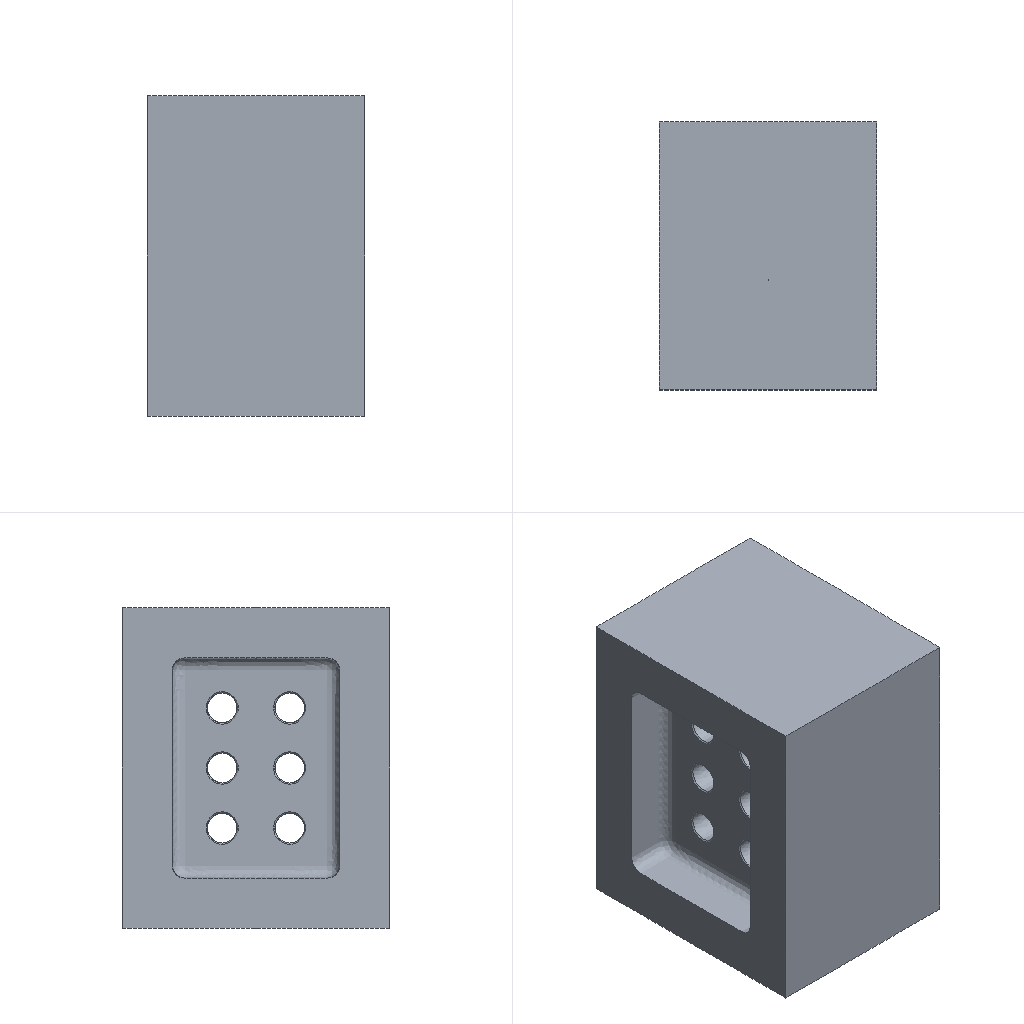Simulation study | ansys workbench
Set-up summary:
category,name,step,type,value,unit,region
solver,ansys_workbench
units,mm-N-s-tonne (MPa),,stated,"/units,MPA"
analysis,LS1,,static
load_step,LS1,LS1,static,nsubst=1; time=1
load_step,LS2,LS2,static,nsubst=1; time=2
mesh,nodes,,,452829
mesh,elements,,,327929
element_type,SOLID187,,,303965
element_type,CONTA174,,,10988
element_type,TARGE170,,,10076
element_type,SURF154,,,2900
material,Structural Steel,,E,200000,tonne s^-2 mm^-1
material,Structural Steel,,nu,0.3
material,Structural Steel,,density,7.85e-09,tonne mm^-3
material,Structural Steel,,conductivity,60.5,tonne mm s^-3 C^-1
material,Structural Steel,,specific_heat,4.34e+08,mm^2 s^-2 C^-1
material,Structural Steel,,cte,1.2e-05,C^-1
material,Structural Steel,,permeability,10000
material,Structural Steel,,resistivity,0.00017,ohm mm
material,mat 29,,E,200000,tonne s^-2 mm^-1
material,mat 29,,nu,0.3
material,mat 29,,density,7.85e-09,tonne mm^-3
material,mat 29,,conductivity,60.5,tonne mm s^-3 C^-1
material,mat 29,,specific_heat,4.34e+08,mm^2 s^-2 C^-1
material,mat 29,,cte,1.2e-05,C^-1
material,mat 29,,permeability,10000
material,mat 29,,resistivity,0.00017,ohm mm
load,Define Force Using Surface Effect Elements,LS1,surface-effect pres face 1,-0.1279,,SURF154 #35
load,Define Force Using Surface Effect Elements,LS1,surface-effect pres face 2,1.43512e-17,,SURF154 #35
load,Define Force Using Surface Effect Elements,LS1,surface-effect pres face 3,6.77494e-18,,SURF154 #35
load,,LS1,force,"6000 [dir=(1, 0, 0) n=6]",,node list
bc,Fixed Supports,model,fixed,[dofs=ALL],,_FIXEDSU
bc,,LS2,prescribed ux,table _FIX [dofs=UX n=6],,node list
contact,Frictional - ? ? ?,,standard (frictionless/frictional),friction=0.2; element=CONTA174
contact,contact 2,,bonded (always),element=CONTA174
contact,contact 3,,bonded (always),element=CONTA174
contact,contact 4,,bonded (always),element=CONTA174
contact,contact 5,,bonded (always),element=CONTA174
contact,contact 6,,bonded (always),element=CONTA174
contact,contact 7,,bonded (always),element=CONTA174
contact,contact 8,,bonded (always),element=CONTA174
contact,contact 9,,bonded (always),element=CONTA174
contact,contact 10,,bonded (always),element=CONTA174
contact,contact 11,,bonded (always),element=CONTA174
contact,contact 12,,bonded (always),element=CONTA174
contact,contact 13,,bonded (always),element=CONTA174
named_set,_FIXEDSU,,node,6188
Ansys APDL input file, long lists of numbers shortened:
/batch
/config,noeldb,1     ! force off writing results to database
*get,_wallstrt,active,,time,wall
! ANSYS input file written by Workbench version 2021 R1
! File used for geometry attach:
/title,__--____ (B5)
! ****** Begin Custom Load Command Snippet ******
/COM, ACT Extensions:
/COM,     LSDYNA, 2021.1
/COM,
! ****** End   Custom Load Command Snippet ******
*DIM,_wb_ProjectScratch_dir,string,248
_wb_ProjectScratch_dir(1) = ''
*DIM,_wb_SolverFiles_dir,string,248
_wb_SolverFiles_dir(1) = ''
*DIM,_wb_userfiles_dir,string,248
_wb_userfiles_dir(1) = ''
/com,--- Data in consistent NMM units. See Solving Units in the help system for more information.
/units,MPA
/nopr
/wb,file,start              !  signify a WB generated input file
/prep7
! Turn off shape checking because checks already performed inside WB mesher.
! See help system for more information.
SHPP,OFF,,NOWARN
/nolist
etcon,set             ! allow ANSYS to choose best KEYOP's for 180x elements, resets any applicable keyopt to MAPDL defaults
/com,*********** Nodes for the whole assembly ***********
nblock,3,,498092
(1i9,3e20.9e3)
        1     2.300000000E+01     1.350000000E+01     7.150000000E+01
! (452810 more lines like these left out)
-1
/com,*********** Nodes for all Remote Points ***********
nblock,3
(1i9,3e20.9e3)
   452812    -2.349999920E+01     1.350120327E+01     6.550000084E+01
! (17 more lines like these left out)
-1
/wb,elem,start            !  set before creation of elements
/com,*********** Elements for Body 1 "__" ***********
et,1,187
eblock,19,solid,,152287
(19i9)
        1        1        1        1        0        0        0        0       10        0   151679   245149   257424   247867   249921   386975   405592   386966   386970
! (304573 more lines like these left out)
-1
/com,*********** Elements for Body 2 "__" ***********
et,2,187
eblock,19,solid,,151678
(19i9)
        2        2        2        2        0        0        0        0       10        0        1    15184    18821    31336    21045   135985   158937   135991   135988
! (303355 more lines like these left out)
-1
/wb,elem,end               !  done creating elements
/com,*********** Send User Defined Coordinate System(s) ***********
csys,0
toffst,273.15,  ! Temperature offset from absolute zero
/com,*********** Set Reference Temperature ***********
tref,22.
/wb,mat,start              !  starting to send materials
/com,*********** Send Materials ***********
Temperature = 'TEMP' ! Temperature
MP,DENS,1,7.85e-09,	! tonne mm^-3
MP,ALPX,1,1.2e-05,	! C^-1
MP,C,1,434000000,	! mm^2 s^-2 C^-1
MP,KXX,1,60.5,	! tonne mm s^-3 C^-1
MP,RSVX,1,0.00017,	! ohm mm
MP,EX,1,200000,	! tonne s^-2 mm^-1
MP,NUXY,1,0.3,
MP,MURX,1,10000,
Temperature = 'TEMP' ! Temperature
MP,DENS,2,7.85e-09,	! tonne mm^-3
MP,ALPX,2,1.2e-05,	! C^-1
MP,C,2,434000000,	! mm^2 s^-2 C^-1
MP,KXX,2,60.5,	! tonne mm s^-3 C^-1
MP,RSVX,2,0.00017,	! ohm mm
MP,EX,2,200000,	! tonne s^-2 mm^-1
MP,NUXY,2,0.3,
MP,MURX,2,10000,
/wb,mat,end                !  done sending materials
!************************* Model Summary ********************
!__,	结构钢,	matid,	1
!__,	结构钢,	matid,	2
!************************* End Model Summary ********************
! get the diagonal of the bounding box. Needed later for other things
*get,_xmin,node,,mnloc,x
*get,_ymin,node,,mnloc,y
*get,_zmin,node,,mnloc,z
*get,_xmax,node,,mxloc,x
*get,_ymax,node,,mxloc,y
*get,_zmax,node,,mxloc,z
_ASMDIAG=(_xmax-_xmin)*(_xmax-_xmin)+(_ymax-_ymin)*(_ymax-_ymin)+(_zmax-_zmin)*(_zmax-_zmin)
_ASMDIAG=SQRT(_ASMDIAG)
/wb,contact,start          !  starting to send contact
/com,*********** Create Contact "摩擦的 - 固体 至 固体" ***********
/com,            Real Constant Set For Above Contact Is 4 & 3
*set,tid,4
*set,cid,3
r,tid
r,cid
et,tid,170
et,cid,174
eblock,10,,,5038
(15i9)
   350529        4        4        4        0   230477   230549   229930   229930   289067   283934   229930   283933
! (5037 more lines like these left out)
-1
eblock,10,,,5038
(15i9)
   355567        3        3        3        0   230477   230549   229930   229930   289067   283934   229930   283933
! (5037 more lines like these left out)
-1
eblock,10,,,5038
(15i9)
   360605        3        4        3        0     3593     4585     4192     4192    56241    61610     4192    56239
! (5037 more lines like these left out)
-1
eblock,10,,,5038
(15i9)
   365643        4        3        4        0     3593     4585     4192     4192    56241    61610     4192    56239
! (5037 more lines like these left out)
-1
keyo,cid,8,2               ! auto create asymmetric contact (from Program Controlled setting)
keyo,cid,10,0              ! adjust contact stiffness each NR iteration (from Program Controlled setting)
keyo,cid,12,0              ! standard contact
mp,mu,cid,0.2       ! unitless
keyo,cid,18,1              ! small sliding turned on by application
keyo,cid,2,0               ! augmented Lagrange (from Program Controlled setting)
keyo,cid,4,0               ! on Gauss point (from Program Controlled setting)
keyo,cid,9,0               ! use real geometry with stepped effects
keyo,cid,7,0               ! No Prediction
rmod,tid,3,1.       ! FKN
rmod,tid,5,0.       ! ICONT
rmod,tid,6,0.       ! PINB
rmod,tid,10,0.      ! CNOF
rmod,tid,12,0.      ! FKT
rmod,tid,36,27      ! WB DSID
rmod,cid,3,1.       ! FKN
rmod,cid,5,0.       ! ICONT
rmod,cid,6,0.       ! PINB
rmod,cid,10,0.      ! CNOF
rmod,cid,12,0.      ! FKT
rmod,cid,36,27      ! WB DSID
nsel,all
esel,all
/wb,contact,end            !  done creating contacts
/golist
/wb,load,start             !  starting to send loads
/com,*********** Fixed Supports ***********
CMBLOCK,_FIXEDSU,NODE,     6188
(8i10)
      1057      1079      1080      1081      1082      1083      1084      1085
! (773 more lines like these left out)
cmsel,s,_FIXEDSU
d,all,all
nsel,all
/com,*********** Create Remote Point "内部远程点" ***********
! -------- Remote Point Used by "循环的 - 固体 至 固体" --------
*set,tid,6
*set,cid,5
et,cid,174
et,tid,170
keyo,tid,2,1               ! Don't fix the pilot node
keyo,tid,4,111111
keyo,cid,12,5              ! Bonded Contact
keyo,cid,4,2               ! Rigid CERIG style load
keyo,cid,2,2               ! MPC style contact
eblock,10,,,64
(15i9)
   370681        5        5        5        0   226617   226628   226629   226629   262476   262567   226629   262477
! (63 more lines like these left out)
-1
*set,_npilot,452812
_npilot40=_npilot
type,tid
mat ,cid
real,cid
tshape,pilo
en,370745,_npilot
tshape
/com,*********** Create Remote Point "内部远程点 2" ***********
! -------- Remote Point Used by "循环的 - 固体 至 固体" --------
*set,tid,8
*set,cid,7
et,cid,174
et,tid,170
keyo,tid,2,1               ! Don't fix the pilot node
keyo,tid,4,111111
keyo,cid,12,5              ! Bonded Contact
keyo,cid,4,2               ! Rigid CERIG style load
keyo,cid,2,2               ! MPC style contact
eblock,10,,,88
(15i9)
   370746        7        7        7        0       20       21     7441     7441    31465    31471     7441    31466
! (87 more lines like these left out)
-1
*set,_npilot,452813
_npilot41=_npilot
type,tid
mat ,cid
real,cid
tshape,pilo
en,370834,_npilot
tshape
/com,*********** Create Remote Point "内部远程点" ***********
! -------- Remote Point Used by "循环的 - 固体 至 固体" --------
*set,tid,10
*set,cid,9
et,cid,174
et,tid,170
keyo,tid,2,1               ! Don't fix the pilot node
keyo,tid,4,111111
keyo,cid,12,5              ! Bonded Contact
keyo,cid,4,2               ! Rigid CERIG style load
keyo,cid,2,2               ! MPC style contact
eblock,10,,,64
(15i9)
   370835        9        9        9        0   226058   226059   226452   226452   257957   257964   226452   257958
! (63 more lines like these left out)
-1
*set,_npilot,452814
_npilot45=_npilot
type,tid
mat ,cid
real,cid
tshape,pilo
en,370899,_npilot
tshape
/com,*********** Create Remote Point "内部远程点 2" ***********
! -------- Remote Point Used by "循环的 - 固体 至 固体" --------
*set,tid,12
*set,cid,11
et,cid,174
et,tid,170
keyo,tid,2,1               ! Don't fix the pilot node
keyo,tid,4,111111
keyo,cid,12,5              ! Bonded Contact
keyo,cid,4,2               ! Rigid CERIG style load
keyo,cid,2,2               ! MPC style contact
eblock,10,,,88
(15i9)
   370900       11       11       11        0      580      701      702      702    35914    36847      702    35915
! (87 more lines like these left out)
-1
*set,_npilot,452815
_npilot47=_npilot
type,tid
mat ,cid
real,cid
tshape,pilo
en,370988,_npilot
tshape
/com,*********** Create Remote Point "内部远程点" ***********
! -------- Remote Point Used by "循环的 - 固体 至 固体" --------
*set,tid,14
*set,cid,13
et,cid,174
et,tid,170
keyo,tid,2,1               ! Don't fix the pilot node
keyo,tid,4,111111
keyo,cid,12,5              ! Bonded Contact
keyo,cid,4,2               ! Rigid CERIG style load
keyo,cid,2,2               ! MPC style contact
eblock,10,,,64
(15i9)
   370989       13       13       13        0   226587   233496   226648   226648   262228   262683   226648   262224
! (63 more lines like these left out)
-1
*set,_npilot,452816
_npilot50=_npilot
type,tid
mat ,cid
real,cid
tshape,pilo
en,371053,_npilot
tshape
/com,*********** Create Remote Point "内部远程点 2" ***********
! -------- Remote Point Used by "循环的 - 固体 至 固体" --------
*set,tid,16
*set,cid,15
et,cid,174
et,tid,170
keyo,tid,2,1               ! Don't fix the pilot node
keyo,tid,4,111111
keyo,cid,12,5              ! Bonded Contact
keyo,cid,4,2               ! Rigid CERIG style load
keyo,cid,2,2               ! MPC style contact
eblock,10,,,88
(15i9)
   371054       15       15       15        0      533      535     7402     7402    35498    35520     7402    35503
! (87 more lines like these left out)
-1
*set,_npilot,452817
_npilot52=_npilot
type,tid
mat ,cid
real,cid
tshape,pilo
en,371142,_npilot
tshape
/com,*********** Create Remote Point "内部远程点" ***********
! -------- Remote Point Used by "循环的 - 固体 至 固体" --------
*set,tid,18
*set,cid,17
et,cid,174
et,tid,170
keyo,tid,2,1               ! Don't fix the pilot node
keyo,tid,4,111111
keyo,cid,12,5              ! Bonded Contact
keyo,cid,4,2               ! Rigid CERIG style load
keyo,cid,2,2               ! MPC style contact
eblock,10,,,64
(15i9)
   371143       17       17       17        0   225993   225994   226486   226486   257544   257552   226486   257545
! (63 more lines like these left out)
-1
*set,_npilot,452818
_npilot55=_npilot
type,tid
mat ,cid
real,cid
tshape,pilo
en,371207,_npilot
tshape
/com,*********** Create Remote Point "内部远程点 2" ***********
! -------- Remote Point Used by "循环的 - 固体 至 固体" --------
*set,tid,20
*set,cid,19
et,cid,174
et,tid,170
keyo,tid,2,1               ! Don't fix the pilot node
keyo,tid,4,111111
keyo,cid,12,5              ! Bonded Contact
keyo,cid,4,2               ! Rigid CERIG style load
keyo,cid,2,2               ! MPC style contact
eblock,10,,,88
(15i9)
   371208       19       19       19        0      606      607     7452     7452    36138    36148     7452    36141
! (87 more lines like these left out)
-1
*set,_npilot,452819
_npilot57=_npilot
type,tid
mat ,cid
real,cid
tshape,pilo
en,371296,_npilot
tshape
/com,*********** Create Remote Point "内部远程点" ***********
! -------- Remote Point Used by "循环的 - 固体 至 固体" --------
*set,tid,22
*set,cid,21
et,cid,174
et,tid,170
keyo,tid,2,1               ! Don't fix the pilot node
keyo,tid,4,111111
keyo,cid,12,5              ! Bonded Contact
keyo,cid,4,2               ! Rigid CERIG style load
keyo,cid,2,2               ! MPC style contact
eblock,10,,,64
(15i9)
   371297       21       21       21        0   226560   226673   226674   226674   262007   262820   226674   262008
! (63 more lines like these left out)
-1
*set,_npilot,452820
_npilot60=_npilot
type,tid
mat ,cid
real,cid
tshape,pilo
en,371361,_npilot
tshape
/com,*********** Create Remote Point "内部远程点 2" ***********
! -------- Remote Point Used by "循环的 - 固体 至 固体" --------
*set,tid,24
*set,cid,23
et,cid,174
et,tid,170
keyo,tid,2,1               ! Don't fix the pilot node
keyo,tid,4,111111
keyo,cid,12,5              ! Bonded Contact
keyo,cid,4,2               ! Rigid CERIG style load
keyo,cid,2,2               ! MPC style contact
eblock,10,,,88
(15i9)
   371362       23       23       23        0      490      672     7471     7471    35135    36672     7471    35139
! (87 more lines like these left out)
-1
*set,_npilot,452821
_npilot62=_npilot
type,tid
mat ,cid
real,cid
tshape,pilo
en,371450,_npilot
tshape
/com,*********** Create Remote Point "内部远程点" ***********
! -------- Remote Point Used by "循环的 - 固体 至 固体" --------
*set,tid,26
*set,cid,25
et,cid,174
et,tid,170
keyo,tid,2,1               ! Don't fix the pilot node
keyo,tid,4,111111
keyo,cid,12,5              ! Bonded Contact
keyo,cid,4,2               ! Rigid CERIG style load
keyo,cid,2,2               ! MPC style contact
eblock,10,,,64
(15i9)
   371451       25       25       25        0   226086   226515   226516   226516   258132   261632   226516   258133
! (63 more lines like these left out)
-1
*set,_npilot,452822
_npilot65=_npilot
type,tid
mat ,cid
real,cid
tshape,pilo
en,371515,_npilot
tshape
/com,*********** Create Remote Point "内部远程点 2" ***********
! -------- Remote Point Used by "循环的 - 固体 至 固体" --------
*set,tid,28
*set,cid,27
et,cid,174
et,tid,170
keyo,tid,2,1               ! Don't fix the pilot node
keyo,tid,4,111111
keyo,cid,12,5              ! Bonded Contact
keyo,cid,4,2               ! Rigid CERIG style load
keyo,cid,2,2               ! MPC style contact
eblock,10,,,88
(15i9)
   371516       27       27       27        0      651     7490      653      653    36542    36557      653    36537
! (87 more lines like these left out)
-1
*set,_npilot,452823
_npilot67=_npilot
type,tid
mat ,cid
real,cid
tshape,pilo
en,371604,_npilot
tshape
/com,*********** Create Beam Connection "___ - __ _ __" ***********
/com,            Real Constant Set For Above Beam Connection Is 29
*set,_bid,29
et,_bid,188
mat,_bid
real,_bid
type,_bid
secnum,_bid
en,350497,452812,452813
sectype,29,beam,csolid
secdata,5.
secoffset,cent
Temperature = 'TEMP' ! Temperature
MP,DENS,29,7.85e-09,	! tonne mm^-3
MP,ALPX,29,1.2e-05,	! C^-1
MP,C,29,434000000,	! mm^2 s^-2 C^-1
MP,KXX,29,60.5,	! tonne mm s^-3 C^-1
MP,RSVX,29,0.00017,	! ohm mm
MP,EX,29,200000,	! tonne s^-2 mm^-1
MP,NUXY,29,0.3,
MP,MURX,29,10000,
/com,*********** Create Beam Connection "___ - __ _ __" ***********
/com,            Real Constant Set For Above Beam Connection Is 30
*set,_bid,30
et,_bid,188
mat,_bid
real,_bid
type,_bid
secnum,_bid
en,350502,452814,452815
sectype,30,beam,csolid
secdata,5.
secoffset,cent
Temperature = 'TEMP' ! Temperature
MP,DENS,30,7.85e-09,	! tonne mm^-3
MP,ALPX,30,1.2e-05,	! C^-1
MP,C,30,434000000,	! mm^2 s^-2 C^-1
MP,KXX,30,60.5,	! tonne mm s^-3 C^-1
MP,RSVX,30,0.00017,	! ohm mm
MP,EX,30,200000,	! tonne s^-2 mm^-1
MP,NUXY,30,0.3,
MP,MURX,30,10000,
/com,*********** Create Beam Connection "___ - __ _ __" ***********
/com,            Real Constant Set For Above Beam Connection Is 31
*set,_bid,31
et,_bid,188
mat,_bid
real,_bid
type,_bid
secnum,_bid
en,350507,452816,452817
sectype,31,beam,csolid
secdata,5.
secoffset,cent
Temperature = 'TEMP' ! Temperature
MP,DENS,31,7.85e-09,	! tonne mm^-3
MP,ALPX,31,1.2e-05,	! C^-1
MP,C,31,434000000,	! mm^2 s^-2 C^-1
MP,KXX,31,60.5,	! tonne mm s^-3 C^-1
MP,RSVX,31,0.00017,	! ohm mm
MP,EX,31,200000,	! tonne s^-2 mm^-1
MP,NUXY,31,0.3,
MP,MURX,31,10000,
/com,*********** Create Beam Connection "___ - __ _ __" ***********
/com,            Real Constant Set For Above Beam Connection Is 32
*set,_bid,32
et,_bid,188
mat,_bid
real,_bid
type,_bid
secnum,_bid
en,350512,452818,452819
sectype,32,beam,csolid
secdata,5.
secoffset,cent
Temperature = 'TEMP' ! Temperature
MP,DENS,32,7.85e-09,	! tonne mm^-3
MP,ALPX,32,1.2e-05,	! C^-1
MP,C,32,434000000,	! mm^2 s^-2 C^-1
MP,KXX,32,60.5,	! tonne mm s^-3 C^-1
MP,RSVX,32,0.00017,	! ohm mm
MP,EX,32,200000,	! tonne s^-2 mm^-1
MP,NUXY,32,0.3,
MP,MURX,32,10000,
/com,*********** Create Beam Connection "___ - __ _ __" ***********
/com,            Real Constant Set For Above Beam Connection Is 33
*set,_bid,33
et,_bid,188
mat,_bid
real,_bid
type,_bid
secnum,_bid
en,350517,452820,452821
sectype,33,beam,csolid
secdata,5.
secoffset,cent
Temperature = 'TEMP' ! Temperature
MP,DENS,33,7.85e-09,	! tonne mm^-3
MP,ALPX,33,1.2e-05,	! C^-1
MP,C,33,434000000,	! mm^2 s^-2 C^-1
MP,KXX,33,60.5,	! tonne mm s^-3 C^-1
MP,RSVX,33,0.00017,	! ohm mm
MP,EX,33,200000,	! tonne s^-2 mm^-1
MP,NUXY,33,0.3,
MP,MURX,33,10000,
/com,*********** Create Beam Connection "___ - __ _ __" ***********
/com,            Real Constant Set For Above Beam Connection Is 34
*set,_bid,34
et,_bid,188
mat,_bid
real,_bid
type,_bid
secnum,_bid
en,350522,452822,452823
sectype,34,beam,csolid
secdata,5.
secoffset,cent
Temperature = 'TEMP' ! Temperature
MP,DENS,34,7.85e-09,	! tonne mm^-3
MP,ALPX,34,1.2e-05,	! C^-1
MP,C,34,434000000,	! mm^2 s^-2 C^-1
MP,KXX,34,60.5,	! tonne mm s^-3 C^-1
MP,RSVX,34,0.00017,	! ohm mm
MP,EX,34,200000,	! tonne s^-2 mm^-1
MP,NUXY,34,0.3,
MP,MURX,34,10000,
/com,*********** Define Force Using Surface Effect Elements ***********
local,12,0,0.,0.,0.,0.,0.,0.
csys,0
et,35,154
eblock,10,,,2900
(15i9)
   371605       35       35       35       12   232476   233277   233096   233096   301242   305167   233096   301239
! (2899 more lines like these left out)
-1
esel,s,type,,35
keyop,35,2,1                ! Apply load in local coordinate system
keyop,35,7,1                ! Use original area so load is constant in large deformation
esel,all
*DIM,_loadvari37x,TABLE,3,1,1,TIME,
! Time values
_loadvari37x(1,0,1) = 0.
_loadvari37x(2,0,1) = 1.
_loadvari37x(3,0,1) = 2.
! Load values
_loadvari37x(1,1,1) = 0.
_loadvari37x(2,1,1) = 0.
_loadvari37x(3,1,1) = -0.1279
*DIM,_loadvari37y,TABLE,3,1,1,TIME,
! Time values
_loadvari37y(1,0,1) = 0.
_loadvari37y(2,0,1) = 1.
_loadvari37y(3,0,1) = 2.
! Load values
_loadvari37y(1,1,1) = 0.
_loadvari37y(2,1,1) = 0.
_loadvari37y(3,1,1) = 1.43512145976393e-017
*DIM,_loadvari37z,TABLE,3,1,1,TIME,
! Time values
_loadvari37z(1,0,1) = 0.
_loadvari37z(2,0,1) = 1.
_loadvari37z(3,0,1) = 2.
! Load values
_loadvari37z(1,1,1) = 0.
_loadvari37z(2,1,1) = 0.
_loadvari37z(3,1,1) = 6.77494355651925e-018
/com,*********** Create Bolt Pretension "_____" ***********
*set,_pretnode,452824
_nbolt69 = 452824               ! that will be the pretension node number
*set,_beame1,350497
*set,_beamn1,452812
*set,_beamn2,452813
_centx = .5*(NX(_beamn1)+NX(_beamn2))
_centy = .5*(NY(_beamn1)+NY(_beamn2))
! (8 more lines like these left out)
local,11,0,_centx,_centy,_centz
nmod,_pretnode,0,0,0,,,,1              ! move pretension node to bolt center, don't update centroid
*get,_nmax,ndmx
_center1=_nmax+1
_center2=_nmax+2
n,_center1,
n,_center2,
*get,_bid,elem,_beame1,ATTR,MAT        ! get the material number of beam connection element
mat,_bid
real,_bid
type,_bid
secnum,_bid
emod,_beame1,2,_center1                ! modify the original beam element to half length
e,_center2,_beamn2                     ! create new beam element to span second half of length
*set,_tid,36
et,_tid,179
type,_tid
real,_tid
mat,_tid
secnum,_tid
e,_center1,_center2,_pretnode          ! directly create pretension element
SECTYPE,_tid,PRETENSION
secdata,_pretnode,_dirx,_diry,_dirz    ! pretension directon set from the 2 beam connection nodes
csys,0
/com,*********** Create Bolt Pretension "_____ 2" ***********
*set,_pretnode,452825
_nbolt70 = 452825               ! that will be the pretension node number
*set,_beame1,350502
*set,_beamn1,452814
*set,_beamn2,452815
_centx = .5*(NX(_beamn1)+NX(_beamn2))
_centy = .5*(NY(_beamn1)+NY(_beamn2))
! (8 more lines like these left out)
local,11,0,_centx,_centy,_centz
nmod,_pretnode,0,0,0,,,,1              ! move pretension node to bolt center, don't update centroid
*get,_nmax,ndmx
_center1=_nmax+1
_center2=_nmax+2
n,_center1,
n,_center2,
*get,_bid,elem,_beame1,ATTR,MAT        ! get the material number of beam connection element
mat,_bid
real,_bid
type,_bid
secnum,_bid
emod,_beame1,2,_center1                ! modify the original beam element to half length
e,_center2,_beamn2                     ! create new beam element to span second half of length
*set,_tid,37
et,_tid,179
type,_tid
real,_tid
mat,_tid
secnum,_tid
e,_center1,_center2,_pretnode          ! directly create pretension element
SECTYPE,_tid,PRETENSION
secdata,_pretnode,_dirx,_diry,_dirz    ! pretension directon set from the 2 beam connection nodes
csys,0
/com,*********** Create Bolt Pretension "_____ 3" ***********
*set,_pretnode,452826
_nbolt71 = 452826               ! that will be the pretension node number
*set,_beame1,350507
*set,_beamn1,452816
*set,_beamn2,452817
_centx = .5*(NX(_beamn1)+NX(_beamn2))
_centy = .5*(NY(_beamn1)+NY(_beamn2))
! (8 more lines like these left out)
local,11,0,_centx,_centy,_centz
nmod,_pretnode,0,0,0,,,,1              ! move pretension node to bolt center, don't update centroid
*get,_nmax,ndmx
_center1=_nmax+1
_center2=_nmax+2
n,_center1,
n,_center2,
*get,_bid,elem,_beame1,ATTR,MAT        ! get the material number of beam connection element
mat,_bid
real,_bid
type,_bid
secnum,_bid
emod,_beame1,2,_center1                ! modify the original beam element to half length
e,_center2,_beamn2                     ! create new beam element to span second half of length
*set,_tid,38
et,_tid,179
type,_tid
real,_tid
mat,_tid
secnum,_tid
e,_center1,_center2,_pretnode          ! directly create pretension element
SECTYPE,_tid,PRETENSION
secdata,_pretnode,_dirx,_diry,_dirz    ! pretension directon set from the 2 beam connection nodes
csys,0
/com,*********** Create Bolt Pretension "_____ 4" ***********
*set,_pretnode,452827
_nbolt72 = 452827               ! that will be the pretension node number
*set,_beame1,350512
*set,_beamn1,452818
*set,_beamn2,452819
_centx = .5*(NX(_beamn1)+NX(_beamn2))
_centy = .5*(NY(_beamn1)+NY(_beamn2))
! (8 more lines like these left out)
local,11,0,_centx,_centy,_centz
nmod,_pretnode,0,0,0,,,,1              ! move pretension node to bolt center, don't update centroid
*get,_nmax,ndmx
_center1=_nmax+1
_center2=_nmax+2
n,_center1,
n,_center2,
*get,_bid,elem,_beame1,ATTR,MAT        ! get the material number of beam connection element
mat,_bid
real,_bid
type,_bid
secnum,_bid
emod,_beame1,2,_center1                ! modify the original beam element to half length
e,_center2,_beamn2                     ! create new beam element to span second half of length
*set,_tid,39
et,_tid,179
type,_tid
real,_tid
mat,_tid
secnum,_tid
e,_center1,_center2,_pretnode          ! directly create pretension element
SECTYPE,_tid,PRETENSION
secdata,_pretnode,_dirx,_diry,_dirz    ! pretension directon set from the 2 beam connection nodes
csys,0
/com,*********** Create Bolt Pretension "_____ 5" ***********
*set,_pretnode,452828
_nbolt73 = 452828               ! that will be the pretension node number
*set,_beame1,350517
*set,_beamn1,452820
*set,_beamn2,452821
_centx = .5*(NX(_beamn1)+NX(_beamn2))
_centy = .5*(NY(_beamn1)+NY(_beamn2))
! (8 more lines like these left out)
local,11,0,_centx,_centy,_centz
nmod,_pretnode,0,0,0,,,,1              ! move pretension node to bolt center, don't update centroid
*get,_nmax,ndmx
_center1=_nmax+1
_center2=_nmax+2
n,_center1,
n,_center2,
*get,_bid,elem,_beame1,ATTR,MAT        ! get the material number of beam connection element
mat,_bid
real,_bid
type,_bid
secnum,_bid
emod,_beame1,2,_center1                ! modify the original beam element to half length
e,_center2,_beamn2                     ! create new beam element to span second half of length
*set,_tid,40
et,_tid,179
type,_tid
real,_tid
mat,_tid
secnum,_tid
e,_center1,_center2,_pretnode          ! directly create pretension element
SECTYPE,_tid,PRETENSION
secdata,_pretnode,_dirx,_diry,_dirz    ! pretension directon set from the 2 beam connection nodes
csys,0
/com,*********** Create Bolt Pretension "_____ 6" ***********
*set,_pretnode,452829
_nbolt74 = 452829               ! that will be the pretension node number
*set,_beame1,350522
*set,_beamn1,452822
*set,_beamn2,452823
_centx = .5*(NX(_beamn1)+NX(_beamn2))
_centy = .5*(NY(_beamn1)+NY(_beamn2))
! (8 more lines like these left out)
local,11,0,_centx,_centy,_centz
nmod,_pretnode,0,0,0,,,,1              ! move pretension node to bolt center, don't update centroid
*get,_nmax,ndmx
_center1=_nmax+1
_center2=_nmax+2
n,_center1,
n,_center2,
*get,_bid,elem,_beame1,ATTR,MAT        ! get the material number of beam connection element
mat,_bid
real,_bid
type,_bid
secnum,_bid
emod,_beame1,2,_center1                ! modify the original beam element to half length
e,_center2,_beamn2                     ! create new beam element to span second half of length
*set,_tid,41
et,_tid,179
type,_tid
real,_tid
mat,_tid
secnum,_tid
e,_center1,_center2,_pretnode          ! directly create pretension element
SECTYPE,_tid,PRETENSION
secdata,_pretnode,_dirx,_diry,_dirz    ! pretension directon set from the 2 beam connection nodes
csys,0
/gst,on,on
fini
*get,_numnode,node,0,count
*get,_numelem,elem,0,count
*get, _MAXELEMNUM, elem, 0, NUM, MAX
*get, _MAXNODENUM, node, 0, NUM, MAX
*get, _MAXELEMTYPE, etyp, 0, NUM, MAX
*get, _MAXREALCONST, real, 0, NUM, MAX
/go
/wb,load,end               !  done creating loads
/com,--- Number of total nodes = %_numnode%
/com,--- Number of contact elements = 23964
/com,--- Number of spring elements = 0
/com,--- Number of bearing elements = 0
/com,--- Number of solid elements = 303965
/com,--- Number of condensed parts = 0
/com,--- Number of total elements = %_numelem%
*get,_wallbsol,active,,time,wall
/com,****************************************************************************
/com,*************************    SOLUTION       ********************************
/com,****************************************************************************
/solu
antype,0                   ! static analysis
_thickRatio=  1     ! Ratio of thick parts in the model
eqsl,pcg,1e-8,,,,,,1
cntr,print,1               ! print out contact info and also make no initial contact an error
dmpoption,emat,no             ! Don't combine emat file for DANSYS
dmpoption,esav,no             ! Don't combine esav file for DANSYS
nldiag,cont,iter           ! print out contact info each equilibrium iteration
rescontrol,define,last,last,,dele	   ! Program Controlled
/com,****************************************************
/com,******************* SOLVE FOR LS 1 OF 2 ****************
esel,s,type,,35
nsle
sfe,all,1,pres,1,%_loadvari37x%
sfe,all,2,pres,1,%_loadvari37y%
sfe,all,3,pres,1,%_loadvari37z%
nsel,all
esel,all
/nopr
/gopr
/nolist
f,452824,fx,1000.
f,452825,fx,1000.
f,452826,fx,1000.
f,452827,fx,1000.
f,452828,fx,1000.
f,452829,fx,1000.
autots,on                  ! Workbench Program Controlled automatic time stepping
nsub,1,10,1                ! due to presence of general nonlinear
time,1.
outres,erase
outres,all,none
outres,nsol,all,
outres,rsol,all
outres,eangl,all
outres,etmp,all
outres,veng,all
outres,strs,all,
outres,epel,all,
outres,eppl,all,
outres,cont,all,
/nopr
esel,s,type,,29
esel,a,type,,30,34
cm,_elmisc,elem
esel,all
/gopr
outres,misc,all,_elmisc
! *********** WB SOLVE COMMAND ***********
! check interactive state
*get,ANSINTER_,active,,int
*if,ANSINTER_,ne,0,then
/eof
*endif
solve
/com *************** Write FE CONNECTORS *********
CEWRITE,file,ce,,INTE
/com,****************************************************
/com,*************** FINISHED SOLVE FOR LS 1 *************
/com,****************************************************
/com,******************* SOLVE FOR LS 2 OF 2 ****************
/nopr
/gopr
/nolist
fdel,452824,all
d,452824,ux,%_FIX%
fdel,452825,all
d,452825,ux,%_FIX%
fdel,452826,all
d,452826,ux,%_FIX%
fdel,452827,all
d,452827,ux,%_FIX%
fdel,452828,all
d,452828,ux,%_FIX%
fdel,452829,all
d,452829,ux,%_FIX%
autots,on                  ! Workbench Program Controlled automatic time stepping
nsub,1,10,1                ! due to presence of general nonlinear
time,2.
outres,erase
outres,all,none
outres,nsol,all,
outres,rsol,all
outres,eangl,all
outres,etmp,all
outres,veng,all
outres,strs,all,
outres,epel,all,
outres,eppl,all,
outres,cont,all,
outres,misc,all,_elmisc
solve
/com,****************************************************
/com,*************** FINISHED SOLVE FOR LS 2 *************
*get,_wallasol,active,,time,wall
/nopr
*get,_numnode,node,0,count
*get,_numelem,elem,0,count
*get, _MAXELEMNUM, elem, 0, NUM, MAX
*get, _MAXNODENUM, node, 0, NUM, MAX,,,INTERNAL
*get, _MAXELEMTYPE, etyp, 0, NUM, MAX
*get, _MAXREALCONST, real, 0, NUM, MAX
/gopr
*get,_PCGITER,active,,solu,cgiter
/post1
xmlo,ENCODING,ISO-8859-1
xmlo,parm
/xml,parm,xml
fini
/gopr
*get,_walldone,active,,time,wall
_preptime=(_wallbsol-_wallstrt)*3600
_solvtime=(_wallasol-_wallbsol)*3600
_posttime=(_walldone-_wallasol)*3600
_totaltim=(_walldone-_wallstrt)*3600
*get,_dlbratio,active,0,solu,dlbr
*get,_combtime,active,0,solu,comb
/com,--- Total number of nodes = %_numnode%
/com,--- Total number of elements = %_numelem%
/com,--- Element load balance ratio = %_dlbratio%
/com,--- Time to combine distributed files = %_combtime%
/wb,file,end               ! done with WB generated input
Results summary:
result,analyses[0].index,,,1
result,analyses[0].system,,,SYS-1
result,analyses[0].deck,,,deck.dat
result,analyses[0].solve_status,,,completed
result,analyses[0].analysis_type,,,static
result,analyses[0].physics,,,mechanical
result,analyses[0].unit_system,,,"NMM: mm, ton, N, s, mV, mA, degC"
result,analyses[0].n_sets,,,2
result,analyses[0].load_steps[0].set,set=1,,1
result,analyses[0].load_steps[0].time_or_freq,set=1,,1
result,analyses[0].load_steps[0].max_displacement_magnitude,set=1,,0.003563
result,analyses[0].load_steps[0].max_von_mises_nodal,set=1,,8.642
result,analyses[0].load_steps[0].reaction_force_sum_xyz[1],set=1,,-1.09759e-09
result,analyses[0].load_steps[0].reaction_force_sum_xyz[2],set=1,,-1.24835e-09
result,analyses[0].load_steps[0].reaction_force_sum_xyz[3],set=1,,1.48652e-09
result,analyses[0].load_steps[1].set,set=2,,2
result,analyses[0].load_steps[1].time_or_freq,set=2,,2
result,analyses[0].load_steps[1].max_displacement_magnitude,set=2,,0.003563
result,analyses[0].load_steps[1].max_von_mises_nodal,set=2,,8.982
result,analyses[0].load_steps[1].reaction_force_sum_xyz[1],set=2,,6996.83
result,analyses[0].load_steps[1].reaction_force_sum_xyz[2],set=2,,1.04567e-09
result,analyses[0].load_steps[1].reaction_force_sum_xyz[3],set=2,,-1.49074e-09
result,geometry_export[0][0],,,.step
result,geometry_export[0][1],,,ok
result,geometry_export[0][2],,,2